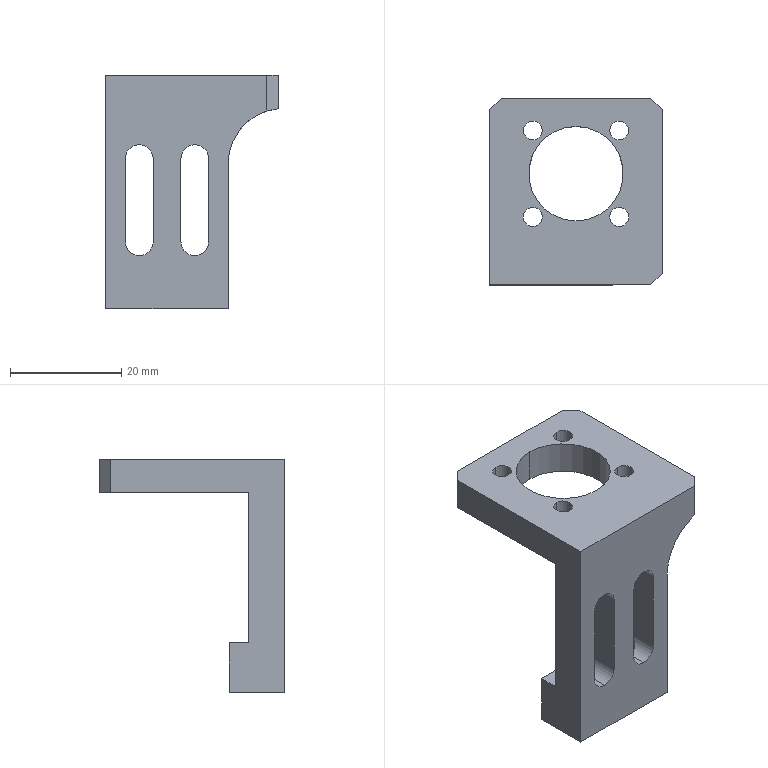NC program | NX | posted with a generic post | part box 31 x 33.478 x 42 mm
Whole program:
N10 G17 G21 G94 G90
(ZLEVEL_PROFILE_COPY , TOOL : D10)
N12 T15 M6
N14 G54
N16 G17 G0 G90 X8.725 Y-22.956 B0. C0. S9500 M3
N18 G43 Z30. H15
N20 Z0.5
N22 G94 G1 Z-1. F1000.
N24 X10.03 Y-22.017
N26 G3 X10.441 Y-21.105 R1.
N28 G1 X9.973 Y-16.451 F3000.
N30 X9.805 Y-15.318
N32 G3 X5.05 Y-11.6 R4.9
N34 G1 X-16.609
N36 X-25.789 Y-11.596
N38 Y-11.597 Z-2.
N40 X-16.609 Y-11.6
N42 X5.05
N44 G2 X9.805 Y-15.318 R4.9
N46 G1 X9.973 Y-16.451
N48 X10.441 Y-21.105
N50 X10.44 Z-3.
N52 X9.972 Y-16.451
N54 X9.805 Y-15.318
N56 G3 X5.05 Y-11.6 R4.9
N58 G1 X-16.609
N60 X-25.789 Y-11.597
N62 Z-4.
N64 X-16.609 Y-11.6
N66 X5.05
N68 G2 X9.805 Y-15.318 R4.9
N70 G1 X9.972 Y-16.451
N72 X10.44 Y-21.105
N74 Z-5.
N76 X9.972 Y-16.451
N78 X9.805 Y-15.318
N80 G3 X5.05 Y-11.6 R4.9
N82 G1 X-16.609
N84 X-25.789 Y-11.597
N86 Z-6.
N88 X-16.609 Y-11.6
N90 X5.05
N92 G2 X9.805 Y-15.318 R4.9
N94 G1 X9.972 Y-16.451
N96 X10.439 Y-21.105
N98 Z-7.
N100 X9.971 Y-16.451
N102 X9.806 Y-15.385
N104 X9.813 Y-15.35
N106 G3 X5.05 Y-11.6 R4.9
N108 G1 X-16.609
N110 X-25.789 Y-11.598
N112 Z-8.
N114 X-16.609 Y-11.6
N116 X5.05
N118 G2 X9.813 Y-15.35 R4.9
N120 G1 X9.806 Y-15.385
N122 X9.971 Y-16.451
N124 X10.439 Y-21.105
N126 Z-9.
N128 X9.971 Y-16.451
N130 X9.813 Y-15.35
N132 G3 X5.05 Y-11.6 R4.9
N134 G1 X-16.609
N136 X-25.789 Y-11.598
N138 Z-10.
N140 X-16.609 Y-11.6
N142 X5.05
N144 G2 X9.813 Y-15.35 R4.9
N146 G1 X9.971 Y-16.451
N148 X10.438 Y-21.105
N150 Z-11.
N152 X9.97 Y-16.451
N154 X9.813 Y-15.35
N156 G3 X5.05 Y-11.6 R4.9
N158 G1 X-16.609
N160 X-25.789 Y-11.599
N162 Z-12.
N164 X-16.609 Y-11.6
N166 X5.05
N168 G2 X9.813 Y-15.35 R4.9
N170 G1 X9.97 Y-16.451
N172 X10.438 Y-21.105
N174 G2 X10.027 Y-22.017 R1.
N176 G1 X8.721 Y-22.956
N178 Z-10.5
N180 G0 Z30.
N182 M5
(ZLEVEL_PROFILE_COPY_COPY , TOOL : D10JING)
N184 T14 M6
N186 G54
N188 G17 G0 G90 X8.387 Y-17.795 B0. C0. S9500 M3
N190 G43 Z30. H14
N192 Z-10.5
N194 G94 G1 Z-12. F1000.
N196 X9.614 Y-16.912
N198 G3 X10.025 Y-16. R1.
N200 X5.05 Y-11.5 R5. F1500.
N202 G1 X-21.
N204 G3 X-21.866 Y-12. R1.
N206 G1 X-22.622 Y-13.309
N208 Z-10.5
N210 G0 Z30.
N212 M5
(ZLEVEL_PROFILE_COPY_1 , TOOL : D4)
N214 T11 M6
N216 G54
N218 G17 G0 G90 X1.177 Y10. B0. C0. S9500 M3
N220 G43 Z30. H11
N222 Z1.5
N224 G94 G1 X-9.176 Z0.957 F1000.
N226 X-9.503 Y9.668 Z0.933
N228 X-9.497 Y9.317 Z0.915
N230 X-9.176 Y9. Z0.891
N232 X6.176 Z0.086
N234 X6.224 Y9.02 Z0.084
N236 X6.475 Y9.266 Z0.065
N238 X6.53 Y9.52 Z0.052
N240 X6.457 Y9.769 Z0.038
N242 X6.188 Y9.996 Z0.02
N244 X6.176 Y10. Z0.019
N246 X-1.5 Z-0.383
N248 X-9. F1650.
N250 G3 X-9.5 Y9.5 R0.5
N252 X-9. Y9. R0.5
N254 G1 X6.
N256 G3 X6.5 Y9.5 R0.5
N258 X6. Y10. R0.5
N260 G1 X-1.5
N262 X-3.375 Z-0.405
N264 X-5.25 Z-0.427
N266 X-7.125 Z-0.448
N268 X-9. Y9.983 Z-0.47
N270 X-9.167 Y9.95 Z-0.472
N272 X-9.244 Y9.917 Z-0.473
N274 X-9.356 Y9.823 Z-0.475
N276 X-9.421 Y9.737 Z-0.476
N278 X-9.47 Y9.602 Z-0.478
N280 X-9.483 Y9.493 Z-0.479
N282 X-9.459 Y9.354 Z-0.481
N284 X-9.416 Y9.254 Z-0.482
N286 X-9.325 Y9.145 Z-0.484
N288 X-9.24 Y9.08 Z-0.485
N290 X-9.148 Y9.042 Z-0.486
N292 X-9. Y9.017 Z-0.488
N294 X-7.125 Y9. Z-0.51
N296 X4.125 Z-0.64
N298 X6. Y9.019 Z-0.662
N300 X6.095 Y9.032 Z-0.663
N302 X6.18 Y9.06 Z-0.664
N304 X6.35 Y9.143 Z-0.666
N306 X6.421 Y9.23 Z-0.668
N308 X6.462 Y9.387 Z-0.669
N310 X6.475 Y9.558 Z-0.671
N312 X6.452 Y9.647 Z-0.673
N314 X6.386 Y9.78 Z-0.674
N316 X6.306 Y9.864 Z-0.676
N318 X6.231 Y9.918 Z-0.677
N320 X6.164 Y9.949 Z-0.678
N322 X6.09 Y9.968 Z-0.679
N324 X6. Y9.981 Z-0.68
N326 X4.125 Y10. Z-0.702
N328 X2.25 Z-0.723
N330 X0.375 Z-0.745
N332 X-1.5 Z-0.767
N334 X-3.375 Z-0.788
N336 X-5.25 Z-0.81
N338 X-7.125 Z-0.832
N340 X-9. Y9.983 Z-0.854
N342 X-9.167 Y9.95 Z-0.856
N344 X-9.244 Y9.917 Z-0.857
N346 X-9.356 Y9.823 Z-0.858
N348 X-9.421 Y9.737 Z-0.86
N350 X-9.47 Y9.602 Z-0.861
N352 X-9.483 Y9.493 Z-0.863
N354 X-9.459 Y9.354 Z-0.864
N356 X-9.416 Y9.254 Z-0.866
N358 X-9.325 Y9.145 Z-0.867
N360 X-9.24 Y9.08 Z-0.869
N362 X-9.148 Y9.042 Z-0.87
N364 X-9. Y9.017 Z-0.871
N366 X-7.125 Y9. Z-0.893
N368 X4.125 Z-1.023
N370 X6. Y9.019 Z-1.045
N372 X6.095 Y9.032 Z-1.046
N374 X6.18 Y9.06 Z-1.047
N376 X6.35 Y9.143 Z-1.05
N378 X6.421 Y9.23 Z-1.051
N380 X6.462 Y9.387 Z-1.053
N382 X6.477 Y9.559 Z-1.055
N384 X6.452 Y9.647 Z-1.056
N386 X6.384 Y9.784 Z-1.058
N388 X6.306 Y9.864 Z-1.059
N390 X6.231 Y9.918 Z-1.06
N392 X6.164 Y9.949 Z-1.061
N394 X6.089 Y9.968 Z-1.062
N396 X6. Y9.981 Z-1.063
N398 X4.125 Y10. Z-1.085
N400 X2.25 Z-1.107
N402 X0.375 Z-1.128
N404 X-1.5 Z-1.15
N406 X-3.375 Z-1.172
N408 X-5.25 Z-1.193
N410 X-7.125 Z-1.215
N412 X-9. Y9.983 Z-1.237
N414 X-9.167 Y9.95 Z-1.239
N416 X-9.244 Y9.917 Z-1.24
N418 X-9.356 Y9.823 Z-1.242
N420 X-9.421 Y9.737 Z-1.243
N422 X-9.47 Y9.602 Z-1.245
N424 X-9.483 Y9.493 Z-1.246
N426 X-9.459 Y9.354 Z-1.248
N428 X-9.416 Y9.254 Z-1.249
N430 X-9.325 Y9.145 Z-1.251
N432 X-9.24 Y9.08 Z-1.252
N434 X-9.148 Y9.042 Z-1.253
N436 X-9. Y9.017 Z-1.255
N438 X-7.125 Y9. Z-1.277
N440 X4.125 Z-1.407
N442 X6. Y9.019 Z-1.428
N444 X6.095 Y9.032 Z-1.43
N446 X6.18 Y9.06 Z-1.431
N448 X6.35 Y9.143 Z-1.433
N450 X6.421 Y9.23 Z-1.434
N452 X6.462 Y9.387 Z-1.436
N454 X6.477 Y9.559 Z-1.438
N456 X6.452 Y9.647 Z-1.439
N458 X6.384 Y9.784 Z-1.441
N460 X6.306 Y9.864 Z-1.442
N462 X6.231 Y9.918 Z-1.444
N464 X6.164 Y9.949
N466 X6.089 Y9.968 Z-1.445
N468 X6. Y9.981 Z-1.446
N470 X4.125 Y10. Z-1.468
N472 X2.25 Z-1.49
N474 X0.375 Z-1.512
N476 X-1.5 Z-1.533
N478 X-3.375 Z-1.555
N480 X-5.25 Z-1.577
N482 X-7.125 Z-1.598
N484 X-9. Y9.983 Z-1.62
N486 X-9.167 Y9.95 Z-1.622
N488 X-9.244 Y9.917 Z-1.623
N490 X-9.357 Y9.825 Z-1.625
N492 X-9.421 Y9.737 Z-1.626
N494 X-9.47 Y9.6 Z-1.628
N496 X-9.483 Y9.493 Z-1.629
N498 X-9.459 Y9.354 Z-1.631
N500 X-9.416 Y9.254 Z-1.632
N502 X-9.325 Y9.145 Z-1.634
N504 X-9.24 Y9.08 Z-1.635
N506 X-9.148 Y9.042 Z-1.636
N508 X-9. Y9.017 Z-1.638
N510 X-7.125 Y9. Z-1.66
N512 X4.125 Z-1.79
N514 X6. Y9.019 Z-1.812
N516 X6.095 Y9.032 Z-1.813
N518 X6.18 Y9.06 Z-1.814
N520 X6.35 Y9.143 Z-1.816
N522 X6.421 Y9.23 Z-1.818
N524 X6.462 Y9.387 Z-1.819
N526 X6.477 Y9.559 Z-1.821
N528 X6.452 Y9.647 Z-1.823
N530 X6.384 Y9.784 Z-1.824
N532 X6.306 Y9.864 Z-1.826
N534 X6.231 Y9.918 Z-1.827
N536 X6.164 Y9.949 Z-1.828
N538 X6.089 Y9.968 Z-1.829
N540 X6. Y9.981 Z-1.83
N542 X4.125 Y10. Z-1.852
N544 X2.25 Z-1.873
N546 X0.375 Z-1.895
N548 X-1.5 Z-1.917
N550 X-3.375 Z-1.938
N552 X-5.25 Z-1.96
N554 X-7.125 Z-1.982
N556 X-9. Y9.983 Z-2.004
N558 X-9.167 Y9.95 Z-2.006
N560 X-9.244 Y9.917 Z-2.007
N562 X-9.357 Y9.825 Z-2.008
N564 X-9.421 Y9.737 Z-2.01
N566 X-9.47 Y9.6 Z-2.011
N568 X-9.483 Y9.493 Z-2.013
N570 X-9.459 Y9.354 Z-2.014
N572 X-9.416 Y9.254 Z-2.016
N574 X-9.325 Y9.145 Z-2.017
N576 X-9.24 Y9.08 Z-2.019
N578 X-9.148 Y9.042 Z-2.02
N580 X-9. Y9.017 Z-2.021
N582 X-7.125 Y9. Z-2.043
N584 X4.125 Z-2.173
N586 X6. Y9.019 Z-2.195
N588 X6.095 Y9.032 Z-2.196
N590 X6.18 Y9.06 Z-2.197
N592 X6.35 Y9.143 Z-2.2
N594 X6.421 Y9.23 Z-2.201
N596 X6.462 Y9.387 Z-2.203
N598 X6.477 Y9.559 Z-2.205
N600 X6.452 Y9.647 Z-2.206
N602 X6.384 Y9.784 Z-2.208
N604 X6.306 Y9.864 Z-2.209
N606 X6.231 Y9.918 Z-2.21
N608 X6.164 Y9.949 Z-2.211
N610 X6.089 Y9.968 Z-2.212
N612 X6. Y9.981 Z-2.213
N614 X4.125 Y10. Z-2.235
N616 X2.25 Z-2.257
N618 X0.375 Z-2.278
N620 X-1.5 Z-2.3
N622 X-3.375 Z-2.322
N624 X-5.25 Z-2.343
N626 X-7.125 Z-2.365
N628 X-9. Y9.983 Z-2.387
N630 X-9.167 Y9.95 Z-2.389
N632 X-9.244 Y9.917 Z-2.39
N634 X-9.357 Y9.825 Z-2.392
N636 X-9.421 Y9.737 Z-2.393
N638 X-9.47 Y9.6 Z-2.395
N640 X-9.483 Y9.493 Z-2.396
N642 X-9.459 Y9.354 Z-2.398
N644 X-9.416 Y9.254 Z-2.399
N646 X-9.325 Y9.145 Z-2.401
N648 X-9.24 Y9.08 Z-2.402
N650 X-9.148 Y9.042 Z-2.403
N652 X-9. Y9.017 Z-2.405
N654 X-7.125 Y9. Z-2.427
N656 X4.125 Z-2.557
N658 X6. Y9.019 Z-2.578
N660 X6.095 Y9.032 Z-2.58
N662 X6.18 Y9.06 Z-2.581
N664 X6.35 Y9.143 Z-2.583
N666 X6.421 Y9.23 Z-2.584
N668 X6.462 Y9.387 Z-2.586
N670 X6.477 Y9.559 Z-2.588
N672 X6.452 Y9.647 Z-2.589
N674 X6.384 Y9.784 Z-2.591
N676 X6.306 Y9.864 Z-2.592
N678 X6.231 Y9.918 Z-2.594
N680 X6.164 Y9.949
N682 X6.089 Y9.968 Z-2.595
N684 X6. Y9.981 Z-2.596
N686 X4.125 Y10. Z-2.618
N688 X2.25 Z-2.64
N690 X0.375 Z-2.662
N692 X-1.5 Z-2.683
N694 X-3.375 Z-2.705
N696 X-5.25 Z-2.727
N698 X-7.125 Z-2.748
N700 X-9. Y9.983 Z-2.77
N702 X-9.167 Y9.95 Z-2.772
N704 X-9.244 Y9.917 Z-2.773
N706 X-9.357 Y9.825 Z-2.775
N708 X-9.421 Y9.737 Z-2.776
N710 X-9.47 Y9.6 Z-2.778
N712 X-9.483 Y9.493 Z-2.779
N714 X-9.459 Y9.354 Z-2.781
N716 X-9.416 Y9.254 Z-2.782
N718 X-9.325 Y9.145 Z-2.784
N720 X-9.24 Y9.08 Z-2.785
N722 X-9.148 Y9.042 Z-2.786
N724 X-9. Y9.017 Z-2.788
N726 X-7.125 Y9. Z-2.81
N728 X4.125 Z-2.94
N730 X6. Y9.019 Z-2.962
N732 X6.095 Y9.032 Z-2.963
N734 X6.18 Y9.06 Z-2.964
N736 X6.35 Y9.143 Z-2.966
N738 X6.421 Y9.23 Z-2.968
N740 X6.462 Y9.387 Z-2.969
N742 X6.477 Y9.559 Z-2.971
N744 X6.452 Y9.647 Z-2.973
N746 X6.384 Y9.784 Z-2.974
N748 X6.306 Y9.864 Z-2.976
N750 X6.231 Y9.918 Z-2.977
N752 X6.164 Y9.949 Z-2.978
N754 X6.09 Y9.968 Z-2.979
N756 X6. Y9.981 Z-2.98
N758 X4.125 Y10. Z-3.002
N760 X2.25 Z-3.023
N762 X0.375 Z-3.045
N764 X-1.5 Z-3.067
N766 X-3.375 Z-3.088
N768 X-5.25 Z-3.11
N770 X-7.125 Z-3.132
N772 X-9. Y9.983 Z-3.154
N774 X-9.167 Y9.95 Z-3.156
N776 X-9.244 Y9.917 Z-3.157
N778 X-9.357 Y9.825 Z-3.158
N780 X-9.421 Y9.737 Z-3.16
N782 X-9.47 Y9.6 Z-3.161
N784 X-9.483 Y9.493 Z-3.163
N786 X-9.459 Y9.354 Z-3.164
N788 X-9.416 Y9.254 Z-3.166
N790 X-9.325 Y9.145 Z-3.167
N792 X-9.24 Y9.08 Z-3.169
N794 X-9.148 Y9.042 Z-3.17
N796 X-9. Y9.017 Z-3.171
N798 X-7.125 Y9. Z-3.193
N800 X4.125 Z-3.323
N802 X6. Y9.019 Z-3.345
N804 X6.095 Y9.032 Z-3.346
N806 X6.18 Y9.06 Z-3.347
N808 X6.35 Y9.143 Z-3.35
N810 X6.421 Y9.23 Z-3.351
N812 X6.462 Y9.387 Z-3.353
N814 X6.477 Y9.559 Z-3.355
N816 X6.452 Y9.647 Z-3.356
N818 X6.384 Y9.784 Z-3.358
N820 X6.306 Y9.864 Z-3.359
N822 X6.231 Y9.918 Z-3.36
N824 X6.164 Y9.949 Z-3.361
N826 X6.09 Y9.968 Z-3.362
N828 X6. Y9.981 Z-3.363
N830 X4.125 Y10. Z-3.385
N832 X2.25 Z-3.407
N834 X0.375 Z-3.428
N836 X-1.5 Z-3.45
N838 X-3.375 Z-3.472
N840 X-5.25 Z-3.493
N842 X-7.125 Z-3.515
N844 X-9. Y9.983 Z-3.537
N846 X-9.167 Y9.95 Z-3.539
N848 X-9.244 Y9.917 Z-3.54
N850 X-9.357 Y9.825 Z-3.542
N852 X-9.421 Y9.737 Z-3.543
N854 X-9.47 Y9.6 Z-3.545
N856 X-9.483 Y9.493 Z-3.546
N858 X-9.459 Y9.354 Z-3.548
N860 X-9.416 Y9.254 Z-3.549
N862 X-9.325 Y9.145 Z-3.551
N864 X-9.24 Y9.08 Z-3.552
N866 X-9.148 Y9.042 Z-3.553
N868 X-9. Y9.017 Z-3.555
N870 X-7.125 Y9. Z-3.577
N872 X4.125 Z-3.707
N874 X6. Y9.019 Z-3.728
N876 X6.095 Y9.032 Z-3.73
N878 X6.18 Y9.06 Z-3.731
N880 X6.35 Y9.143 Z-3.733
N882 X6.421 Y9.23 Z-3.734
N884 X6.462 Y9.387 Z-3.736
N886 X6.477 Y9.559 Z-3.738
N888 X6.452 Y9.647 Z-3.739
N890 X6.384 Y9.784 Z-3.741
N892 X6.306 Y9.864 Z-3.742
N894 X6.231 Y9.918 Z-3.744
N896 X6.164 Y9.949
N898 X6.09 Y9.968 Z-3.745
N900 X6. Y9.981 Z-3.746
N902 X4.125 Y10. Z-3.768
N904 X2.25 Z-3.79
N906 X0.375 Z-3.812
N908 X-1.5 Z-3.833
N910 X-3.375 Z-3.855
N912 X-5.25 Z-3.877
N914 X-7.125 Z-3.898
N916 X-9. Y9.983 Z-3.92
N918 X-9.167 Y9.95 Z-3.922
N920 X-9.244 Y9.917 Z-3.923
N922 X-9.357 Y9.825 Z-3.925
N924 X-9.421 Y9.737 Z-3.926
N926 X-9.47 Y9.6 Z-3.928
N928 X-9.483 Y9.493 Z-3.929
N930 X-9.459 Y9.354 Z-3.931
N932 X-9.416 Y9.254 Z-3.932
N934 X-9.325 Y9.145 Z-3.934
N936 X-9.24 Y9.08 Z-3.935
N938 X-9.148 Y9.042 Z-3.936
N940 X-9. Y9.017 Z-3.938
N942 X-7.125 Y9. Z-3.96
N944 X4.125 Z-4.09
N946 X6. Y9.019 Z-4.112
N948 X6.095 Y9.032 Z-4.113
N950 X6.18 Y9.06 Z-4.114
N952 X6.35 Y9.143 Z-4.116
N954 X6.421 Y9.23 Z-4.118
N956 X6.462 Y9.387 Z-4.119
N958 X6.477 Y9.559 Z-4.121
N960 X6.452 Y9.647 Z-4.123
N962 X6.384 Y9.784 Z-4.124
N964 X6.306 Y9.864 Z-4.126
N966 X6.231 Y9.918 Z-4.127
N968 X6.164 Y9.949 Z-4.128
N970 X6.09 Y9.968 Z-4.129
N972 X6. Y9.981 Z-4.13
N974 X4.125 Y10. Z-4.152
N976 X2.25 Z-4.173
N978 X0.375 Z-4.195
N980 X-1.5 Z-4.217
N982 X-3.375 Z-4.238
N984 X-5.25 Z-4.26
N986 X-7.125 Z-4.282
N988 X-9. Y9.983 Z-4.304
N990 X-9.167 Y9.95 Z-4.306
N992 X-9.244 Y9.917 Z-4.307
N994 X-9.357 Y9.825 Z-4.308
N996 X-9.421 Y9.737 Z-4.31
N998 X-9.47 Y9.6 Z-4.311
N1000 X-9.483 Y9.493 Z-4.313
N1002 X-9.459 Y9.354 Z-4.314
N1004 X-9.416 Y9.254 Z-4.316
N1006 X-9.325 Y9.145 Z-4.317
N1008 X-9.24 Y9.08 Z-4.319
N1010 X-9.148 Y9.042 Z-4.32
N1012 X-9. Y9.017 Z-4.321
N1014 X-7.125 Y9. Z-4.343
N1016 X4.125 Z-4.473
N1018 X6. Y9.019 Z-4.495
N1020 X6.095 Y9.032 Z-4.496
N1022 X6.18 Y9.06 Z-4.497
N1024 X6.35 Y9.143 Z-4.5
N1026 X6.421 Y9.23 Z-4.501
N1028 X6.462 Y9.387 Z-4.503
N1030 X6.477 Y9.559 Z-4.505
N1032 X6.452 Y9.647 Z-4.506
N1034 X6.384 Y9.784 Z-4.508
N1036 X6.306 Y9.864 Z-4.509
N1038 X6.231 Y9.918 Z-4.51
N1040 X6.164 Y9.949 Z-4.511
N1042 X6.09 Y9.968 Z-4.512
N1044 X6. Y9.981 Z-4.513
N1046 X4.125 Y10. Z-4.535
N1048 X2.25 Z-4.557
N1050 X0.375 Z-4.578
N1052 X-1.5 Z-4.6
N1054 X-3.375 Z-4.622
N1056 X-5.25 Z-4.643
N1058 X-7.125 Z-4.665
N1060 X-9. Y9.983 Z-4.687
N1062 X-9.167 Y9.95 Z-4.689
N1064 X-9.244 Y9.917 Z-4.69
N1066 X-9.357 Y9.825 Z-4.692
N1068 X-9.421 Y9.737 Z-4.693
N1070 X-9.47 Y9.6 Z-4.695
N1072 X-9.483 Y9.493 Z-4.696
N1074 X-9.458 Y9.354 Z-4.698
N1076 X-9.416 Y9.254 Z-4.699
N1078 X-9.325 Y9.145 Z-4.701
N1080 X-9.24 Y9.08 Z-4.702
N1082 X-9.148 Y9.042 Z-4.703
N1084 X-9. Y9.017 Z-4.705
N1086 X-7.125 Y9. Z-4.727
N1088 X4.125 Z-4.857
N1090 X6. Y9.019 Z-4.878
N1092 X6.095 Y9.032 Z-4.88
N1094 X6.18 Y9.06 Z-4.881
N1096 X6.35 Y9.143 Z-4.883
N1098 X6.421 Y9.23 Z-4.884
N1100 X6.462 Y9.387 Z-4.886
N1102 X6.477 Y9.559 Z-4.888
N1104 X6.452 Y9.647 Z-4.889
N1106 X6.384 Y9.784 Z-4.891
N1108 X6.306 Y9.864 Z-4.892
N1110 X6.231 Y9.918 Z-4.894
N1112 X6.164 Y9.949
N1114 X6.09 Y9.968 Z-4.895
N1116 X6. Y9.981 Z-4.896
N1118 X4.125 Y10. Z-4.918
N1120 X2.25 Z-4.94
N1122 X0.375 Z-4.962
N1124 X-1.5 Z-4.983
N1126 X-3.375 Z-5.005
N1128 X-5.25 Z-5.027
N1130 X-7.125 Z-5.048
N1132 X-9. Y9.983 Z-5.07
N1134 X-9.167 Y9.95 Z-5.072
N1136 X-9.244 Y9.917 Z-5.073
N1138 X-9.357 Y9.825 Z-5.075
N1140 X-9.421 Y9.737 Z-5.076
N1142 X-9.47 Y9.6 Z-5.078
N1144 X-9.483 Y9.493 Z-5.079
N1146 X-9.458 Y9.354 Z-5.081
N1148 X-9.416 Y9.254 Z-5.082
N1150 X-9.325 Y9.145 Z-5.084
N1152 X-9.24 Y9.08 Z-5.085
N1154 X-9.148 Y9.042 Z-5.086
N1156 X-9. Y9.017 Z-5.088
N1158 X-7.125 Y9. Z-5.11
N1160 X4.125 Z-5.24
N1162 X6. Y9.019 Z-5.262
N1164 X6.095 Y9.032 Z-5.263
N1166 X6.18 Y9.06 Z-5.264
N1168 X6.35 Y9.143 Z-5.266
N1170 X6.421 Y9.23 Z-5.268
N1172 X6.462 Y9.387 Z-5.269
N1174 X6.477 Y9.559 Z-5.271
N1176 X6.452 Y9.647 Z-5.273
N1178 X6.384 Y9.783 Z-5.274
N1180 X6.306 Y9.864 Z-5.276
N1182 X6.231 Y9.918 Z-5.277
N1184 X6.164 Y9.949 Z-5.278
N1186 X6.09 Y9.968 Z-5.279
N1188 X6. Y9.981 Z-5.28
N1190 X4.125 Y10. Z-5.302
N1192 X2.25 Z-5.323
N1194 X0.375 Z-5.345
N1196 X-1.5 Z-5.367
N1198 X-3.375 Z-5.388
N1200 X-5.25 Z-5.41
N1202 X-7.125 Z-5.432
N1204 X-9. Y9.983 Z-5.454
N1206 X-9.167 Y9.95 Z-5.456
N1208 X-9.244 Y9.917 Z-5.457
N1210 X-9.357 Y9.825 Z-5.458
N1212 X-9.421 Y9.737 Z-5.46
N1214 X-9.47 Y9.6 Z-5.461
N1216 X-9.483 Y9.493 Z-5.463
N1218 X-9.458 Y9.354 Z-5.464
N1220 X-9.416 Y9.254 Z-5.466
N1222 X-9.325 Y9.145 Z-5.467
N1224 X-9.24 Y9.08 Z-5.469
N1226 X-9.148 Y9.042 Z-5.47
N1228 X-9. Y9.017 Z-5.471
N1230 X-7.125 Y9. Z-5.493
N1232 X4.125 Z-5.623
N1234 X6. Y9.019 Z-5.645
N1236 X6.095 Y9.032 Z-5.646
N1238 X6.18 Y9.06 Z-5.647
N1240 X6.35 Y9.143 Z-5.65
N1242 X6.421 Y9.23 Z-5.651
N1244 X6.462 Y9.387 Z-5.653
N1246 X6.477 Y9.559 Z-5.655
N1248 X6.452 Y9.647 Z-5.656
N1250 X6.384 Y9.783 Z-5.658
N1252 X6.306 Y9.864 Z-5.659
N1254 X6.231 Y9.918 Z-5.66
N1256 X6.164 Y9.949 Z-5.661
N1258 X6.09 Y9.968 Z-5.662
N1260 X6. Y9.981 Z-5.663
N1262 X4.125 Y10. Z-5.685
N1264 X2.25 Z-5.707
N1266 X0.375 Z-5.728
N1268 X-1.5 Z-5.75
N1270 X-3.375 Z-5.772
N1272 X-5.25 Z-5.793
N1274 X-7.125 Z-5.815
N1276 X-9. Y9.983 Z-5.837
N1278 X-9.167 Y9.95 Z-5.839
N1280 X-9.244 Y9.917 Z-5.84
N1282 X-9.357 Y9.825 Z-5.842
N1284 X-9.421 Y9.737 Z-5.843
N1286 X-9.47 Y9.6 Z-5.845
N1288 X-9.483 Y9.493 Z-5.846
N1290 X-9.458 Y9.354 Z-5.848
N1292 X-9.416 Y9.254 Z-5.849
N1294 X-9.325 Y9.145 Z-5.851
N1296 X-9.24 Y9.08 Z-5.852
N1298 X-9.148 Y9.042 Z-5.853
N1300 X-9. Y9.017 Z-5.855
N1302 X-7.125 Y9. Z-5.877
N1304 X4.125 Z-6.007
N1306 X6. Y9.019 Z-6.028
N1308 X6.095 Y9.032 Z-6.03
N1310 X6.18 Y9.06 Z-6.031
N1312 X6.35 Y9.143 Z-6.033
N1314 X6.421 Y9.23 Z-6.034
N1316 X6.462 Y9.387 Z-6.036
N1318 X6.477 Y9.559 Z-6.038
N1320 X6.452 Y9.647 Z-6.039
N1322 X6.384 Y9.783 Z-6.041
N1324 X6.306 Y9.864 Z-6.042
N1326 X6.231 Y9.918 Z-6.044
N1328 X6.164 Y9.949
N1330 X6.09 Y9.968 Z-6.045
N1332 X6. Y9.981 Z-6.046
N1334 X4.125 Y10. Z-6.068
N1336 X2.25 Z-6.09
N1338 X0.375 Z-6.112
N1340 X-1.5 Z-6.133
N1342 X-3.375 Z-6.155
N1344 X-5.25 Z-6.177
N1346 X-7.125 Z-6.198
N1348 X-9. Y9.983 Z-6.22
N1350 X-9.167 Y9.95 Z-6.222
N1352 X-9.244 Y9.917 Z-6.223
N1354 X-9.357 Y9.825 Z-6.225
N1356 X-9.421 Y9.737 Z-6.226
N1358 X-9.47 Y9.6 Z-6.228
N1360 X-9.483 Y9.493 Z-6.229
N1362 X-9.458 Y9.354 Z-6.231
N1364 X-9.416 Y9.254 Z-6.232
N1366 X-9.325 Y9.145 Z-6.234
N1368 X-9.24 Y9.08 Z-6.235
N1370 X-9.148 Y9.042 Z-6.236
N1372 X-9. Y9.017 Z-6.238
N1374 X-7.125 Y9. Z-6.26
N1376 X4.125 Z-6.39
N1378 X6. Y9.019 Z-6.412
N1380 X6.095 Y9.032 Z-6.413
N1382 X6.18 Y9.06 Z-6.414
N1384 X6.35 Y9.143 Z-6.416
N1386 X6.421 Y9.23 Z-6.418
N1388 X6.462 Y9.387 Z-6.419
N1390 X6.477 Y9.559 Z-6.422
N1392 X6.452 Y9.647 Z-6.423
N1394 X6.384 Y9.783 Z-6.424
N1396 X6.306 Y9.864 Z-6.426
N1398 X6.231 Y9.918 Z-6.427
N1400 X6.164 Y9.949 Z-6.428
N1402 X6.09 Y9.968 Z-6.429
N1404 X6. Y9.981 Z-6.43
N1406 X4.125 Y10. Z-6.452
N1408 X2.25 Z-6.473
N1410 X0.375 Z-6.495
N1412 X-1.5 Z-6.517
N1414 X-3.375 Z-6.538
N1416 X-5.25 Z-6.56
N1418 X-7.125 Z-6.582
N1420 X-9. Y9.983 Z-6.604
N1422 X-9.167 Y9.95 Z-6.606
N1424 X-9.244 Y9.917 Z-6.607
N1426 X-9.357 Y9.825 Z-6.608
N1428 X-9.421 Y9.737 Z-6.61
N1430 X-9.47 Y9.6 Z-6.611
N1432 X-9.483 Y9.493 Z-6.613
N1434 X-9.458 Y9.354 Z-6.614
N1436 X-9.416 Y9.254 Z-6.616
N1438 X-9.325 Y9.145 Z-6.617
N1440 X-9.24 Y9.08 Z-6.619
N1442 X-9.148 Y9.042 Z-6.62
N1444 X-9. Y9.017 Z-6.621
N1446 X-7.125 Y9. Z-6.643
N1448 X4.125 Z-6.773
N1450 X6. Y9.019 Z-6.795
N1452 X6.113 Y9.036 Z-6.797
N1454 X6.18 Y9.06
N1456 X6.288 Y9.12 Z-6.799
N1458 X6.334 Y9.159 Z-6.8
N1460 X6.429 Y9.288 Z-6.802
N1462 X6.462 Y9.387 Z-6.803
N1464 X6.475 Y9.545 Z-6.805
N1466 X6.452 Y9.647 Z-6.806
N1468 X6.389 Y9.776 Z-6.808
N1470 X6.306 Y9.864 Z-6.809
N1472 X6.232 Y9.917 Z-6.81
N1474 X6.164 Y9.949 Z-6.811
N1476 X6.09 Y9.968 Z-6.812
N1478 X6. Y9.981 Z-6.813
N1480 X4.125 Y10. Z-6.835
N1482 X2.25 Z-6.857
N1484 X0.375 Z-6.878
N1486 X-1.5 Z-6.9
N1488 X-9.
N1490 G3 X-9.5 Y9.5 R0.5
N1492 X-9. Y9. R0.5
N1494 G1 X6.
N1496 G3 X6.5 Y9.5 R0.5
N1498 X6. Y10. R0.5
N1500 G1 X-1.5
N1502 Z-5.4
N1504 G0 Z30.
N1506 X-4.177 Y-1.
N1508 Z1.5
N1510 G1 X6.176 Z0.957 F1000.
N1512 X6.188 Y-0.996
N1514 X6.457 Y-0.769 Z0.938
N1516 X6.53 Y-0.52 Z0.925
N1518 X6.475 Y-0.266 Z0.911
N1520 X6.224 Y-0.02 Z0.893
N1522 X6.176 Y0. Z0.89
N1524 X-9.176 Z0.085
N1526 X-9.497 Y-0.317 Z0.062
N1528 X-9.503 Y-0.668 Z0.043
N1530 X-9.176 Y-1. Z0.019
N1532 X-1.5 Z-0.383
N1534 X6. F1650.
N1536 G3 X6.5 Y-0.5 R0.5
N1538 X6. Y0. R0.5
N1540 G1 X-9.
N1542 G3 X-9.5 Y-0.5 R0.5
N1544 X-9. Y-1. R0.5
N1546 G1 X-1.5
N1548 X4.125 Z-0.448
N1550 X6. Y-0.981 Z-0.47
N1552 X6.107 Y-0.966 Z-0.471
N1554 X6.164 Y-0.949 Z-0.472
N1556 X6.255 Y-0.906 Z-0.473
N1558 X6.307 Y-0.864 Z-0.474
N1560 X6.475 Y-0.655 Z-0.477
N1562 X6.497 Y-0.55 Z-0.479
N1564 X6.462 Y-0.387 Z-0.481
N1566 X6.396 Y-0.237 Z-0.483
N1568 X6.334 Y-0.159 Z-0.484
N1570 X6.262 Y-0.098 Z-0.485
N1572 X6.18 Y-0.06 Z-0.486
N1574 X6.09 Y-0.033 Z-0.487
N1576 X6. Y-0.019 Z-0.488
N1578 X4.125 Y0. Z-0.51
N1580 X-7.125 Z-0.64
N1582 X-9. Y-0.017 Z-0.662
N1584 X-9.164 Y-0.048 Z-0.664
N1586 X-9.24 Y-0.08 Z-0.665
N1588 X-9.352 Y-0.171 Z-0.667
N1590 X-9.416 Y-0.254 Z-0.668
N1592 X-9.47 Y-0.387 Z-0.669
N1594 X-9.483 Y-0.493 Z-0.671
N1596 X-9.462 Y-0.64 Z-0.673
N1598 X-9.421 Y-0.737 Z-0.674
N1600 X-9.329 Y-0.853 Z-0.676
N1602 X-9.244 Y-0.917 Z-0.677
N1604 X-9.148 Y-0.958 Z-0.678
N1606 X-9. Y-0.983 Z-0.68
N1608 X-7.125 Y-1. Z-0.702
N1610 X-1.5 Z-0.767
N1612 X4.125 Z-0.832
N1614 X6. Y-0.981 Z-0.854
N1616 X6.107 Y-0.966 Z-0.855
N1618 X6.164 Y-0.949 Z-0.856
N1620 X6.255 Y-0.906 Z-0.857
N1622 X6.306 Y-0.864 Z-0.858
N1624 X6.475 Y-0.655 Z-0.861
N1626 X6.497 Y-0.55 Z-0.862
N1628 X6.462 Y-0.387 Z-0.864
N1630 X6.396 Y-0.237 Z-0.866
N1632 X6.334 Y-0.159 Z-0.867
N1634 X6.262 Y-0.098 Z-0.868
N1636 X6.18 Y-0.06 Z-0.869
N1638 X6.09 Y-0.033 Z-0.87
N1640 X6. Y-0.019 Z-0.872
N1642 X4.125 Y0. Z-0.893
N1644 X-7.125 Z-1.023
N1646 X-9. Y-0.017 Z-1.045
N1648 X-9.164 Y-0.048 Z-1.047
N1650 X-9.24 Y-0.08 Z-1.048
N1652 X-9.352 Y-0.171 Z-1.05
N1654 X-9.416 Y-0.254 Z-1.051
N1656 X-9.47 Y-0.387 Z-1.053
N1658 X-9.483 Y-0.493 Z-1.054
N1660 X-9.462 Y-0.64 Z-1.056
N1662 X-9.421 Y-0.737 Z-1.057
N1664 X-9.329 Y-0.853 Z-1.059
N1666 X-9.244 Y-0.917 Z-1.06
N1668 X-9.148 Y-0.958 Z-1.061
N1670 X-9. Y-0.983 Z-1.063
N1672 X-7.125 Y-1. Z-1.085
N1674 X-1.5 Z-1.15
N1676 X4.125 Z-1.215
N1678 X6. Y-0.981 Z-1.237
N1680 X6.107 Y-0.966 Z-1.238
N1682 X6.164 Y-0.949 Z-1.239
N1684 X6.255 Y-0.906 Z-1.24
N1686 X6.306 Y-0.864 Z-1.241
N1688 X6.475 Y-0.655 Z-1.244
N1690 X6.497 Y-0.55 Z-1.245
N1692 X6.462 Y-0.387 Z-1.247
N1694 X6.396 Y-0.237 Z-1.249
N1696 X6.334 Y-0.159 Z-1.25
N1698 X6.262 Y-0.098 Z-1.252
N1700 X6.18 Y-0.06 Z-1.253
N1702 X6.09 Y-0.033 Z-1.254
N1704 X6. Y-0.019 Z-1.255
N1706 X4.125 Y0. Z-1.277
N1708 X-7.125 Z-1.407
N1710 X-9. Y-0.017 Z-1.429
N1712 X-9.164 Y-0.048 Z-1.43
N1714 X-9.24 Y-0.08 Z-1.431
N1716 X-9.352 Y-0.171 Z-1.433
N1718 X-9.416 Y-0.254 Z-1.434
N1720 X-9.47 Y-0.387 Z-1.436
N1722 X-9.483 Y-0.493 Z-1.437
N1724 X-9.462 Y-0.64 Z-1.439
N1726 X-9.421 Y-0.737 Z-1.44
N1728 X-9.329 Y-0.853 Z-1.442
N1730 X-9.244 Y-0.917 Z-1.443
N1732 X-9.148 Y-0.958 Z-1.445
N1734 X-9. Y-0.983 Z-1.446
N1736 X-7.125 Y-1. Z-1.468
N1738 X-1.5 Z-1.533
N1740 X4.125 Z-1.598
N1742 X6. Y-0.981 Z-1.62
N1744 X6.107 Y-0.966 Z-1.621
N1746 X6.164 Y-0.949 Z-1.622
N1748 X6.255 Y-0.906 Z-1.623
N1750 X6.306 Y-0.864 Z-1.624
N1752 X6.475 Y-0.655 Z-1.627
N1754 X6.497 Y-0.55 Z-1.629
N1756 X6.462 Y-0.387 Z-1.631
N1758 X6.396 Y-0.237 Z-1.633
N1760 X6.334 Y-0.159 Z-1.634
N1762 X6.262 Y-0.098 Z-1.635
N1764 X6.18 Y-0.06 Z-1.636
N1766 X6.09 Y-0.033 Z-1.637
N1768 X6. Y-0.019 Z-1.638
N1770 X4.125 Y0. Z-1.66
N1772 X-7.125 Z-1.79
N1774 X-9. Y-0.017 Z-1.812
N1776 X-9.164 Y-0.048 Z-1.814
N1778 X-9.24 Y-0.08 Z-1.815
N1780 X-9.352 Y-0.171 Z-1.817
N1782 X-9.416 Y-0.254 Z-1.818
N1784 X-9.47 Y-0.387 Z-1.819
N1786 X-9.483 Y-0.493 Z-1.821
N1788 X-9.462 Y-0.64 Z-1.823
N1790 X-9.421 Y-0.737 Z-1.824
N1792 X-9.329 Y-0.853 Z-1.826
N1794 X-9.244 Y-0.917 Z-1.827
N1796 X-9.148 Y-0.958 Z-1.828
N1798 X-9. Y-0.983 Z-1.83
N1800 X-7.125 Y-1. Z-1.852
N1802 X-1.5 Z-1.917
N1804 X4.125 Z-1.982
N1806 X6. Y-0.981 Z-2.004
N1808 X6.107 Y-0.966 Z-2.005
N1810 X6.164 Y-0.949 Z-2.006
N1812 X6.255 Y-0.906 Z-2.007
N1814 X6.306 Y-0.864 Z-2.008
N1816 X6.475 Y-0.655 Z-2.011
N1818 X6.497 Y-0.55 Z-2.012
N1820 X6.462 Y-0.387 Z-2.014
N1822 X6.396 Y-0.237 Z-2.016
N1824 X6.334 Y-0.159 Z-2.017
N1826 X6.262 Y-0.098 Z-2.018
N1828 X6.18 Y-0.06 Z-2.019
N1830 X6.09 Y-0.033 Z-2.02
N1832 X6. Y-0.019 Z-2.022
N1834 X4.125 Y0. Z-2.043
N1836 X-7.125 Z-2.173
N1838 X-9. Y-0.017 Z-2.195
N1840 X-9.164 Y-0.048 Z-2.197
N1842 X-9.24 Y-0.08 Z-2.198
N1844 X-9.352 Y-0.171 Z-2.2
N1846 X-9.416 Y-0.254 Z-2.201
N1848 X-9.47 Y-0.387 Z-2.203
N1850 X-9.483 Y-0.493 Z-2.204
N1852 X-9.462 Y-0.64 Z-2.206
N1854 X-9.421 Y-0.737 Z-2.207
N1856 X-9.329 Y-0.853 Z-2.209
N1858 X-9.244 Y-0.917 Z-2.21
N1860 X-9.149 Y-0.957 Z-2.211
N1862 X-9. Y-0.983 Z-2.213
N1864 X-7.125 Y-1. Z-2.235
N1866 X-1.5 Z-2.3
N1868 X4.125 Z-2.365
N1870 X6. Y-0.981 Z-2.387
N1872 X6.107 Y-0.966 Z-2.388
N1874 X6.164 Y-0.949 Z-2.389
N1876 X6.255 Y-0.906 Z-2.39
N1878 X6.306 Y-0.864 Z-2.391
N1880 X6.475 Y-0.655 Z-2.394
N1882 X6.497 Y-0.55 Z-2.395
N1884 X6.462 Y-0.387 Z-2.397
N1886 X6.396 Y-0.237 Z-2.399
N1888 X6.334 Y-0.159 Z-2.4
N1890 X6.262 Y-0.098 Z-2.402
N1892 X6.18 Y-0.06 Z-2.403
N1894 X6.09 Y-0.033 Z-2.404
N1896 X6. Y-0.019 Z-2.405
N1898 X4.125 Y0. Z-2.427
N1900 X-7.125 Z-2.557
N1902 X-9. Y-0.017 Z-2.579
N1904 X-9.164 Y-0.048 Z-2.58
N1906 X-9.24 Y-0.08 Z-2.581
N1908 X-9.352 Y-0.171 Z-2.583
N1910 X-9.416 Y-0.254 Z-2.584
N1912 X-9.47 Y-0.387 Z-2.586
N1914 X-9.483 Y-0.493 Z-2.587
N1916 X-9.462 Y-0.64 Z-2.589
N1918 X-9.421 Y-0.737 Z-2.59
N1920 X-9.329 Y-0.853 Z-2.592
N1922 X-9.244 Y-0.917 Z-2.593
N1924 X-9.149 Y-0.957 Z-2.595
N1926 X-9. Y-0.983 Z-2.596
N1928 X-7.125 Y-1. Z-2.618
N1930 X-1.5 Z-2.683
N1932 X4.125 Z-2.748
N1934 X6. Y-0.981 Z-2.77
N1936 X6.107 Y-0.966 Z-2.771
N1938 X6.164 Y-0.949 Z-2.772
N1940 X6.255 Y-0.906 Z-2.773
N1942 X6.306 Y-0.864 Z-2.774
N1944 X6.475 Y-0.655 Z-2.777
N1946 X6.497 Y-0.55 Z-2.779
N1948 X6.462 Y-0.387 Z-2.781
N1950 X6.396 Y-0.237 Z-2.783
N1952 X6.334 Y-0.159 Z-2.784
N1954 X6.262 Y-0.098 Z-2.785
N1956 X6.18 Y-0.06 Z-2.786
N1958 X6.09 Y-0.033 Z-2.787
N1960 X6. Y-0.019 Z-2.788
N1962 X4.125 Y0. Z-2.81
N1964 X-7.125 Z-2.94
N1966 X-9. Y-0.017 Z-2.962
N1968 X-9.164 Y-0.048 Z-2.964
N1970 X-9.24 Y-0.08 Z-2.965
N1972 X-9.352 Y-0.171 Z-2.967
N1974 X-9.416 Y-0.254 Z-2.968
N1976 X-9.47 Y-0.387 Z-2.969
N1978 X-9.483 Y-0.493 Z-2.971
N1980 X-9.462 Y-0.64 Z-2.973
N1982 X-9.421 Y-0.737 Z-2.974
N1984 X-9.329 Y-0.853 Z-2.976
N1986 X-9.244 Y-0.917 Z-2.977
N1988 X-9.149 Y-0.957 Z-2.978
N1990 X-9. Y-0.983 Z-2.98
N1992 X-7.125 Y-1. Z-3.002
N1994 X-1.5 Z-3.067
N1996 X4.125 Z-3.132
N1998 X6. Y-0.981 Z-3.154
N2000 X6.107 Y-0.966 Z-3.155
N2002 X6.164 Y-0.949 Z-3.156
N2004 X6.255 Y-0.906 Z-3.157
N2006 X6.306 Y-0.864 Z-3.158
N2008 X6.475 Y-0.655 Z-3.161
N2010 X6.497 Y-0.55 Z-3.162
N2012 X6.462 Y-0.387 Z-3.164
N2014 X6.396 Y-0.237 Z-3.166
N2016 X6.334 Y-0.159 Z-3.167
N2018 X6.262 Y-0.098 Z-3.168
N2020 X6.18 Y-0.06 Z-3.169
N2022 X6.09 Y-0.033 Z-3.17
N2024 X6. Y-0.019 Z-3.172
N2026 X4.125 Y0. Z-3.193
N2028 X-7.125 Z-3.323
N2030 X-9. Y-0.017 Z-3.345
N2032 X-9.164 Y-0.048 Z-3.347
N2034 X-9.24 Y-0.08 Z-3.348
N2036 X-9.353 Y-0.17 Z-3.35
N2038 X-9.416 Y-0.254 Z-3.351
N2040 X-9.471 Y-0.39 Z-3.353
N2042 X-9.483 Y-0.493 Z-3.354
N2044 X-9.462 Y-0.64 Z-3.356
N2046 X-9.421 Y-0.737 Z-3.357
N2048 X-9.329 Y-0.853 Z-3.359
N2050 X-9.244 Y-0.917 Z-3.36
N2052 X-9.149 Y-0.957 Z-3.361
N2054 X-9. Y-0.983 Z-3.363
N2056 X-7.125 Y-1. Z-3.385
N2058 X-1.5 Z-3.45
N2060 X4.125 Z-3.515
N2062 X6. Y-0.981 Z-3.537
N2064 X6.107 Y-0.966 Z-3.538
N2066 X6.164 Y-0.949 Z-3.539
N2068 X6.255 Y-0.906 Z-3.54
N2070 X6.306 Y-0.864 Z-3.541
N2072 X6.475 Y-0.655 Z-3.544
N2074 X6.497 Y-0.55 Z-3.545
N2076 X6.462 Y-0.387 Z-3.547
N2078 X6.396 Y-0.237 Z-3.549
N2080 X6.334 Y-0.159 Z-3.55
N2082 X6.262 Y-0.098 Z-3.552
N2084 X6.18 Y-0.06 Z-3.553
N2086 X6.09 Y-0.033 Z-3.554
N2088 X6. Y-0.019 Z-3.555
N2090 X4.125 Y0. Z-3.577
N2092 X-7.125 Z-3.707
N2094 X-9. Y-0.017 Z-3.729
N2096 X-9.164 Y-0.048 Z-3.73
N2098 X-9.24 Y-0.08 Z-3.731
N2100 X-9.353 Y-0.17 Z-3.733
N2102 X-9.416 Y-0.254 Z-3.734
N2104 X-9.471 Y-0.39 Z-3.736
N2106 X-9.483 Y-0.493 Z-3.737
N2108 X-9.462 Y-0.64 Z-3.739
N2110 X-9.421 Y-0.737 Z-3.74
N2112 X-9.329 Y-0.853 Z-3.742
N2114 X-9.244 Y-0.917 Z-3.743
N2116 X-9.149 Y-0.957 Z-3.745
N2118 X-9. Y-0.983 Z-3.746
N2120 X-7.125 Y-1. Z-3.768
N2122 X-1.5 Z-3.833
N2124 X4.125 Z-3.898
N2126 X6. Y-0.981 Z-3.92
N2128 X6.107 Y-0.966 Z-3.921
N2130 X6.164 Y-0.949 Z-3.922
N2132 X6.255 Y-0.906 Z-3.923
N2134 X6.306 Y-0.864 Z-3.924
N2136 X6.475 Y-0.655 Z-3.927
N2138 X6.497 Y-0.55 Z-3.929
N2140 X6.462 Y-0.387 Z-3.931
N2142 X6.396 Y-0.237 Z-3.933
N2144 X6.334 Y-0.159 Z-3.934
N2146 X6.262 Y-0.098 Z-3.935
N2148 X6.18 Y-0.06 Z-3.936
N2150 X6.09 Y-0.033 Z-3.937
N2152 X6. Y-0.019 Z-3.938
N2154 X4.125 Y0. Z-3.96
N2156 X-7.125 Z-4.09
N2158 X-9. Y-0.017 Z-4.112
N2160 X-9.164 Y-0.048 Z-4.114
N2162 X-9.24 Y-0.08 Z-4.115
N2164 X-9.353 Y-0.17 Z-4.117
N2166 X-9.416 Y-0.254 Z-4.118
N2168 X-9.471 Y-0.39 Z-4.12
N2170 X-9.483 Y-0.493 Z-4.121
N2172 X-9.462 Y-0.64 Z-4.123
N2174 X-9.421 Y-0.737 Z-4.124
N2176 X-9.329 Y-0.853 Z-4.126
N2178 X-9.244 Y-0.917 Z-4.127
N2180 X-9.149 Y-0.957 Z-4.128
N2182 X-9. Y-0.983 Z-4.13
N2184 X-7.125 Y-1. Z-4.152
N2186 X-1.5 Z-4.217
N2188 X4.125 Z-4.282
N2190 X6. Y-0.981 Z-4.304
N2192 X6.107 Y-0.966 Z-4.305
N2194 X6.164 Y-0.949 Z-4.306
N2196 X6.255 Y-0.906 Z-4.307
N2198 X6.306 Y-0.864 Z-4.308
N2200 X6.475 Y-0.655 Z-4.311
N2202 X6.497 Y-0.55 Z-4.312
N2204 X6.462 Y-0.387 Z-4.314
N2206 X6.396 Y-0.237 Z-4.316
N2208 X6.334 Y-0.159 Z-4.317
N2210 X6.262 Y-0.098 Z-4.318
N2212 X6.18 Y-0.06 Z-4.319
N2214 X6.09 Y-0.033 Z-4.32
N2216 X6. Y-0.019 Z-4.322
N2218 X4.125 Y0. Z-4.343
N2220 X-7.125 Z-4.473
N2222 X-9. Y-0.017 Z-4.495
N2224 X-9.164 Y-0.048 Z-4.497
N2226 X-9.24 Y-0.08 Z-4.498
N2228 X-9.353 Y-0.17 Z-4.5
N2230 X-9.416 Y-0.254 Z-4.501
N2232 X-9.471 Y-0.39 Z-4.503
N2234 X-9.483 Y-0.493 Z-4.504
N2236 X-9.462 Y-0.64 Z-4.506
N2238 X-9.421 Y-0.737 Z-4.507
N2240 X-9.329 Y-0.853 Z-4.509
N2242 X-9.244 Y-0.917 Z-4.51
N2244 X-9.149 Y-0.957 Z-4.511
N2246 X-9. Y-0.983 Z-4.513
N2248 X-7.125 Y-1. Z-4.535
N2250 X-1.5 Z-4.6
N2252 X4.125 Z-4.665
N2254 X6. Y-0.981 Z-4.687
N2256 X6.107 Y-0.966 Z-4.688
N2258 X6.164 Y-0.949 Z-4.689
N2260 X6.255 Y-0.906 Z-4.69
N2262 X6.306 Y-0.864 Z-4.691
N2264 X6.475 Y-0.655 Z-4.694
N2266 X6.497 Y-0.55 Z-4.695
N2268 X6.462 Y-0.387 Z-4.697
N2270 X6.396 Y-0.237 Z-4.699
N2272 X6.334 Y-0.159 Z-4.7
N2274 X6.262 Y-0.098 Z-4.702
N2276 X6.18 Y-0.06 Z-4.703
N2278 X6.09 Y-0.033 Z-4.704
N2280 X6. Y-0.019 Z-4.705
N2282 X4.125 Y0. Z-4.727
N2284 X-7.125 Z-4.857
N2286 X-9. Y-0.017 Z-4.879
N2288 X-9.164 Y-0.048 Z-4.88
N2290 X-9.24 Y-0.08 Z-4.881
N2292 X-9.353 Y-0.17 Z-4.883
N2294 X-9.416 Y-0.254 Z-4.884
N2296 X-9.471 Y-0.39 Z-4.886
N2298 X-9.483 Y-0.493 Z-4.887
N2300 X-9.462 Y-0.64 Z-4.889
N2302 X-9.421 Y-0.737 Z-4.89
N2304 X-9.329 Y-0.853 Z-4.892
N2306 X-9.244 Y-0.917 Z-4.893
N2308 X-9.149 Y-0.957 Z-4.895
N2310 X-9. Y-0.983 Z-4.896
N2312 X-7.125 Y-1. Z-4.918
N2314 X-1.5 Z-4.983
N2316 X4.125 Z-5.048
N2318 X6. Y-0.981 Z-5.07
N2320 X6.107 Y-0.966 Z-5.071
N2322 X6.164 Y-0.949 Z-5.072
N2324 X6.255 Y-0.906 Z-5.073
N2326 X6.306 Y-0.864 Z-5.074
N2328 X6.475 Y-0.655 Z-5.077
N2330 X6.497 Y-0.55 Z-5.079
N2332 X6.462 Y-0.387 Z-5.081
N2334 X6.396 Y-0.237 Z-5.083
N2336 X6.334 Y-0.159 Z-5.084
N2338 X6.262 Y-0.098 Z-5.085
N2340 X6.18 Y-0.06 Z-5.086
N2342 X6.09 Y-0.033 Z-5.087
N2344 X6. Y-0.019 Z-5.088
N2346 X4.125 Y0. Z-5.11
N2348 X-7.125 Z-5.24
N2350 X-9. Y-0.017 Z-5.262
N2352 X-9.164 Y-0.048 Z-5.264
N2354 X-9.24 Y-0.08 Z-5.265
N2356 X-9.353 Y-0.17 Z-5.267
N2358 X-9.416 Y-0.254 Z-5.268
N2360 X-9.471 Y-0.39 Z-5.27
N2362 X-9.483 Y-0.493 Z-5.271
N2364 X-9.462 Y-0.64 Z-5.273
N2366 X-9.421 Y-0.737 Z-5.274
N2368 X-9.329 Y-0.853 Z-5.276
N2370 X-9.244 Y-0.917 Z-5.277
N2372 X-9.149 Y-0.957 Z-5.278
N2374 X-9. Y-0.983 Z-5.28
N2376 X-7.125 Y-1. Z-5.302
N2378 X-1.5 Z-5.367
N2380 X4.125 Z-5.432
N2382 X6. Y-0.981 Z-5.454
N2384 X6.107 Y-0.966 Z-5.455
N2386 X6.164 Y-0.949 Z-5.456
N2388 X6.255 Y-0.906 Z-5.457
N2390 X6.306 Y-0.864 Z-5.458
N2392 X6.475 Y-0.655 Z-5.461
N2394 X6.497 Y-0.55 Z-5.462
N2396 X6.462 Y-0.387 Z-5.464
N2398 X6.396 Y-0.237 Z-5.466
N2400 X6.334 Y-0.159 Z-5.467
N2402 X6.262 Y-0.098 Z-5.468
N2404 X6.18 Y-0.06 Z-5.469
N2406 X6.09 Y-0.033 Z-5.47
N2408 X6. Y-0.019 Z-5.472
N2410 X4.125 Y0. Z-5.493
N2412 X-7.125 Z-5.623
N2414 X-9. Y-0.017 Z-5.645
N2416 X-9.164 Y-0.048 Z-5.647
N2418 X-9.24 Y-0.08 Z-5.648
N2420 X-9.353 Y-0.17 Z-5.65
N2422 X-9.416 Y-0.254 Z-5.651
N2424 X-9.471 Y-0.39 Z-5.653
N2426 X-9.483 Y-0.493 Z-5.654
N2428 X-9.462 Y-0.64 Z-5.656
N2430 X-9.421 Y-0.737 Z-5.657
N2432 X-9.329 Y-0.853 Z-5.659
N2434 X-9.244 Y-0.917 Z-5.66
N2436 X-9.149 Y-0.957 Z-5.661
N2438 X-9. Y-0.983 Z-5.663
N2440 X-7.125 Y-1. Z-5.685
N2442 X-1.5 Z-5.75
N2444 X4.125 Z-5.815
N2446 X6. Y-0.981 Z-5.837
N2448 X6.107 Y-0.966 Z-5.838
N2450 X6.164 Y-0.949 Z-5.839
N2452 X6.255 Y-0.906 Z-5.84
N2454 X6.306 Y-0.864 Z-5.841
N2456 X6.475 Y-0.655 Z-5.844
N2458 X6.497 Y-0.55 Z-5.845
N2460 X6.462 Y-0.387 Z-5.847
N2462 X6.396 Y-0.237 Z-5.849
N2464 X6.334 Y-0.159 Z-5.85
N2466 X6.262 Y-0.098 Z-5.852
N2468 X6.18 Y-0.06 Z-5.853
N2470 X6.09 Y-0.033 Z-5.854
N2472 X6. Y-0.019 Z-5.855
N2474 X4.125 Y0. Z-5.877
N2476 X-7.125 Z-6.007
N2478 X-9. Y-0.017 Z-6.029
N2480 X-9.164 Y-0.048 Z-6.03
N2482 X-9.24 Y-0.08 Z-6.031
N2484 X-9.353 Y-0.17 Z-6.033
N2486 X-9.416 Y-0.254 Z-6.034
N2488 X-9.47 Y-0.39 Z-6.036
N2490 X-9.483 Y-0.493 Z-6.037
N2492 X-9.462 Y-0.64 Z-6.039
N2494 X-9.421 Y-0.737 Z-6.04
N2496 X-9.329 Y-0.853 Z-6.042
N2498 X-9.244 Y-0.917 Z-6.043
N2500 X-9.149 Y-0.957 Z-6.045
N2502 X-9. Y-0.983 Z-6.046
N2504 X-7.125 Y-1. Z-6.068
N2506 X-1.5 Z-6.133
N2508 X4.125 Z-6.198
N2510 X6. Y-0.981 Z-6.22
N2512 X6.107 Y-0.966 Z-6.221
N2514 X6.164 Y-0.949 Z-6.222
N2516 X6.255 Y-0.906 Z-6.223
N2518 X6.306 Y-0.864 Z-6.224
N2520 X6.475 Y-0.655 Z-6.227
N2522 X6.497 Y-0.55 Z-6.229
N2524 X6.462 Y-0.387 Z-6.231
N2526 X6.396 Y-0.237 Z-6.233
N2528 X6.334 Y-0.159 Z-6.234
N2530 X6.262 Y-0.098 Z-6.235
N2532 X6.18 Y-0.06 Z-6.236
N2534 X6.09 Y-0.033 Z-6.237
N2536 X6. Y-0.019 Z-6.238
N2538 X4.125 Y0. Z-6.26
N2540 X-7.125 Z-6.39
N2542 X-9. Y-0.017 Z-6.412
N2544 X-9.164 Y-0.048 Z-6.414
N2546 X-9.24 Y-0.08 Z-6.415
N2548 X-9.353 Y-0.17 Z-6.417
N2550 X-9.416 Y-0.254 Z-6.418
N2552 X-9.47 Y-0.39 Z-6.42
N2554 X-9.483 Y-0.493 Z-6.421
N2556 X-9.462 Y-0.64 Z-6.423
N2558 X-9.421 Y-0.737 Z-6.424
N2560 X-9.329 Y-0.853 Z-6.426
N2562 X-9.244 Y-0.917 Z-6.427
N2564 X-9.149 Y-0.957 Z-6.428
N2566 X-9. Y-0.983 Z-6.43
N2568 X-7.125 Y-1. Z-6.452
N2570 X-1.5 Z-6.517
N2572 X4.125 Z-6.582
N2574 X6. Y-0.981 Z-6.604
N2576 X6.107 Y-0.966 Z-6.605
N2578 X6.164 Y-0.949 Z-6.606
N2580 X6.262 Y-0.902 Z-6.607
N2582 X6.306 Y-0.864 Z-6.608
N2584 X6.419 Y-0.728 Z-6.61
N2586 X6.452 Y-0.647 Z-6.611
N2588 X6.476 Y-0.49 Z-6.613
N2590 X6.462 Y-0.387 Z-6.614
N2592 X6.405 Y-0.25 Z-6.616
N2594 X6.334 Y-0.159 Z-6.617
N2596 X6.262 Y-0.098 Z-6.618
N2598 X6.18 Y-0.06 Z-6.619
N2600 X6.09 Y-0.033 Z-6.62
N2602 X6. Y-0.019 Z-6.622
N2604 X4.125 Y0. Z-6.643
N2606 X-7.125 Z-6.773
N2608 X-9. Y-0.017 Z-6.795
N2610 X-9.164 Y-0.048 Z-6.797
N2612 X-9.24 Y-0.08 Z-6.798
N2614 X-9.353 Y-0.17 Z-6.8
N2616 X-9.416 Y-0.254 Z-6.801
N2618 X-9.47 Y-0.39 Z-6.803
N2620 X-9.483 Y-0.493 Z-6.804
N2622 X-9.462 Y-0.64 Z-6.806
N2624 X-9.421 Y-0.737 Z-6.807
N2626 X-9.329 Y-0.853 Z-6.809
N2628 X-9.244 Y-0.917 Z-6.81
N2630 X-9.149 Y-0.957 Z-6.811
N2632 X-9. Y-0.983 Z-6.813
N2634 X-7.125 Y-1. Z-6.835
N2636 X-1.5 Z-6.9
N2638 X6.
N2640 G3 X6.5 Y-0.5 R0.5
N2642 X6. Y0. R0.5
N2644 G1 X-9.
N2646 G3 X-9.5 Y-0.5 R0.5
N2648 X-9. Y-1. R0.5
N2650 G1 X-1.5
N2652 Z-5.4
N2654 G0 Z30.
N2656 M5
(PLANAR_MILL_COPY_COPY_1 , TOOL : D6A45)
N2658 T01 M6
N2660 G54
N2662 G17 G0 G90 X-0.634 Y10.6 B0. C0. S9500 M3
N2664 G43 Z30. H1
N2666 Z0.5
N2668 G94 G1 Z-1. F1250.
N2670 G3 X-1.5 Y11.1 R1.
N2672 G1 X-9.
N2674 G3 X-10.6 Y9.5 R1.6
N2676 X-9. Y7.9 R1.6
N2678 G1 X6.
N2680 G3 X7.6 Y9.5 R1.6
N2682 X6. Y11.1 R1.6
N2684 G1 X-1.5
N2686 G3 X-2.366 Y10.6 R1.
N2688 G1 Z0.5
N2690 G0 Z30.
N2692 X-0.866 Y16.9
N2694 Z0.5
N2696 G1 Z-1.
N2698 G3 X0. Y16.4 R1.
N2700 G1 X21.
N2702 G2 X21.9 Y15.5 R0.9
N2704 G1 Y-15.5
N2706 G2 X21. Y-16.4 R0.9
N2708 G1 X15.
N2710 G2 X14.11 Y-15.635 R0.9
N2712 G1 X13.964 Y-14.676
N2714 X13.724 Y-13.748
N2716 G3 X5.05 Y-7.4 R9.1
N2718 G1 X-21.
N2720 G2 X-21.9 Y-6.5 R0.9
N2722 G1 Y15.5
N2724 G2 X-21. Y16.4 R0.9
N2726 G1 X0.
N2728 G3 X0.866 Y16.9 R1.
N2730 G1 Z0.5
N2732 G0 Z30.
N2734 X-0.634 Y0.6
N2736 Z0.5
N2738 G1 Z-1.
N2740 G3 X-1.5 Y1.1 R1.
N2742 G1 X-9.
N2744 G3 X-10.6 Y-0.5 R1.6
N2746 X-9. Y-2.1 R1.6
N2748 G1 X6.
N2750 G3 X7.6 Y-0.5 R1.6
N2752 X6. Y1.1 R1.6
N2754 G1 X-1.5
N2756 G3 X-2.366 Y0.6 R1.
N2758 G1 Z0.5
N2760 G0 Z30.
(PLANAR_MILL_COPY_COPY_1_COPY , TOOL : D6A45)
N2762 X21.866 Y-16.5
N2764 Z-1.
N2766 G1 Z-2.5
N2768 G3 X21. Y-16. R1.
N2770 G1 X14.59
N2772 G3 X13.723 Y-16.5 R1.
N2774 G1 Z-1.
N2776 G0 Z30.
N2778 M5
N2780 M2